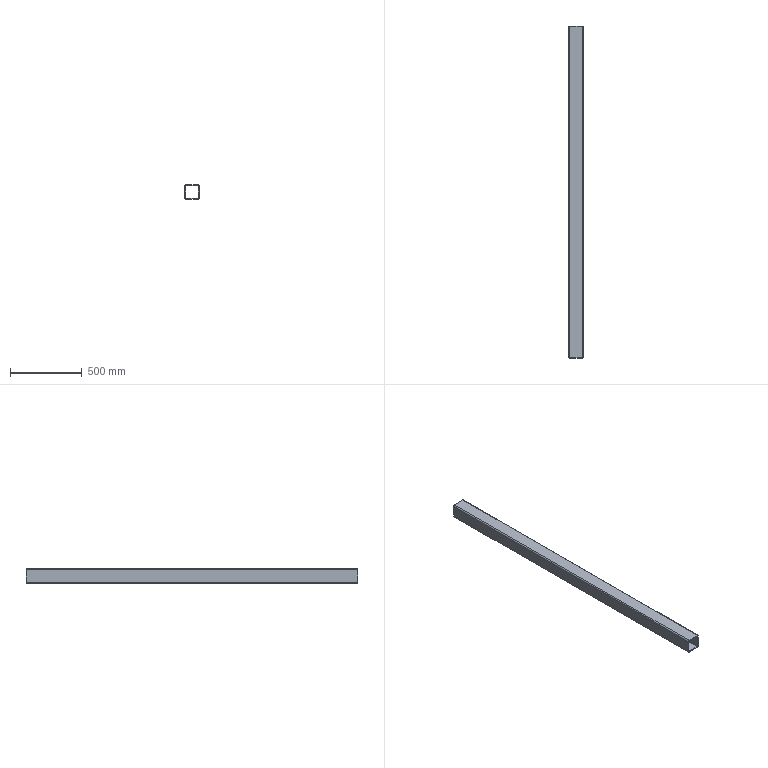Part | SolidWorks | features Extrusion 1 | 1 solid | 18 faces | box 100 x 2320 x 100 mm | volume 5433615 mm3 | plane 10 | cylinder 8 | commonest cylinder face diameters 12.6 x4 15.75 x4
STEP:
#1=CARTESIAN_POINT('',(100.,2320.,-90.6));
#2=VERTEX_POINT('',#1);
#3=CARTESIAN_POINT('',(92.125,2320.,-98.475));
#4=VERTEX_POINT('',#3);
#5=CARTESIAN_POINT('',(92.125,2320.,-90.6));
#6=DIRECTION('',(0.,1.,0.));
#7=DIRECTION('',(0.,0.,1.));
#8=AXIS2_PLACEMENT_3D('',#5,#6,#7);
#9=CIRCLE('',#8,7.875);
#10=EDGE_CURVE('',#2,#4,#9,.T.);
#11=ORIENTED_EDGE('',*,*,#10,.T.);
#12=CARTESIAN_POINT('',(7.875,2320.,-98.475));
#13=VERTEX_POINT('',#12);
#14=CARTESIAN_POINT('',(92.125,2320.,-98.475));
#15=DIRECTION('',(-1.,0.,0.));
#16=VECTOR('',#15,1000.);
#17=LINE('',#14,#16);
#18=EDGE_CURVE('',#4,#13,#17,.T.);
#19=ORIENTED_EDGE('',*,*,#18,.T.);
#20=CARTESIAN_POINT('',(0.,2320.,-90.6));
#21=VERTEX_POINT('',#20);
#22=CARTESIAN_POINT('',(7.875,2320.,-90.6));
#23=DIRECTION('',(0.,1.,0.));
#24=DIRECTION('',(0.,0.,1.));
#25=AXIS2_PLACEMENT_3D('',#22,#23,#24);
#26=CIRCLE('',#25,7.875);
#27=EDGE_CURVE('',#13,#21,#26,.T.);
#28=ORIENTED_EDGE('',*,*,#27,.T.);
#29=CARTESIAN_POINT('',(0.,2320.,-6.35));
#30=VERTEX_POINT('',#29);
#31=CARTESIAN_POINT('',(0.,2320.,-6.35));
#32=DIRECTION('',(0.,0.,1.));
#33=VECTOR('',#32,1000.);
#34=LINE('',#31,#33);
#35=EDGE_CURVE('',#21,#30,#34,.T.);
#36=ORIENTED_EDGE('',*,*,#35,.T.);
#37=CARTESIAN_POINT('',(7.875,2320.,1.525));
#38=VERTEX_POINT('',#37);
#39=CARTESIAN_POINT('',(7.875,2320.,-6.35));
#40=DIRECTION('',(0.,1.,0.));
#41=DIRECTION('',(0.,0.,1.));
#42=AXIS2_PLACEMENT_3D('',#39,#40,#41);
#43=CIRCLE('',#42,7.875);
#44=EDGE_CURVE('',#30,#38,#43,.T.);
#45=ORIENTED_EDGE('',*,*,#44,.T.);
#46=CARTESIAN_POINT('',(92.125,2320.,1.525));
#47=VERTEX_POINT('',#46);
#48=CARTESIAN_POINT('',(7.875,2320.,1.525));
#49=DIRECTION('',(1.,0.,0.));
#50=VECTOR('',#49,1000.);
#51=LINE('',#48,#50);
#52=EDGE_CURVE('',#38,#47,#51,.T.);
#53=ORIENTED_EDGE('',*,*,#52,.T.);
#54=CARTESIAN_POINT('',(100.,2320.,-6.35));
#55=VERTEX_POINT('',#54);
#56=CARTESIAN_POINT('',(92.125,2320.,-6.35));
#57=DIRECTION('',(0.,1.,0.));
#58=DIRECTION('',(0.,0.,1.));
#59=AXIS2_PLACEMENT_3D('',#56,#57,#58);
#60=CIRCLE('',#59,7.875);
#61=EDGE_CURVE('',#47,#55,#60,.T.);
#62=ORIENTED_EDGE('',*,*,#61,.T.);
#63=CARTESIAN_POINT('',(100.,2320.,-90.6));
#64=DIRECTION('',(0.,0.,-1.));
#65=VECTOR('',#64,1000.);
#66=LINE('',#63,#65);
#67=EDGE_CURVE('',#55,#2,#66,.T.);
#68=ORIENTED_EDGE('',*,*,#67,.T.);
#69=EDGE_LOOP('',(#11,#19,#28,#36,#45,#53,#62,#68));
#70=FACE_OUTER_BOUND('',#69,.T.);
#71=CARTESIAN_POINT('',(6.3,2320.,-85.875));
#72=VERTEX_POINT('',#71);
#73=CARTESIAN_POINT('',(6.3,2320.,-11.075));
#74=VERTEX_POINT('',#73);
#75=CARTESIAN_POINT('',(6.3,2320.,-11.075));
#76=DIRECTION('',(0.,0.,1.));
#77=VECTOR('',#76,1000.);
#78=LINE('',#75,#77);
#79=EDGE_CURVE('',#72,#74,#78,.T.);
#80=ORIENTED_EDGE('',*,*,#79,.F.);
#81=CARTESIAN_POINT('',(12.6,2320.,-92.175));
#82=VERTEX_POINT('',#81);
#83=CARTESIAN_POINT('',(12.6,2320.,-85.875));
#84=DIRECTION('',(0.,1.,0.));
#85=DIRECTION('',(0.,0.,1.));
#86=AXIS2_PLACEMENT_3D('',#83,#84,#85);
#87=CIRCLE('',#86,6.3);
#88=EDGE_CURVE('',#82,#72,#87,.T.);
#89=ORIENTED_EDGE('',*,*,#88,.F.);
#90=CARTESIAN_POINT('',(87.4,2320.,-92.175));
#91=VERTEX_POINT('',#90);
#92=CARTESIAN_POINT('',(87.4,2320.,-92.175));
#93=DIRECTION('',(-1.,0.,0.));
#94=VECTOR('',#93,1000.);
#95=LINE('',#92,#94);
#96=EDGE_CURVE('',#91,#82,#95,.T.);
#97=ORIENTED_EDGE('',*,*,#96,.F.);
#98=CARTESIAN_POINT('',(93.7,2320.,-85.875));
#99=VERTEX_POINT('',#98);
#100=CARTESIAN_POINT('',(87.4,2320.,-85.875));
#101=DIRECTION('',(0.,1.,0.));
#102=DIRECTION('',(0.,0.,1.));
#103=AXIS2_PLACEMENT_3D('',#100,#101,#102);
#104=CIRCLE('',#103,6.3);
#105=EDGE_CURVE('',#99,#91,#104,.T.);
#106=ORIENTED_EDGE('',*,*,#105,.F.);
#107=CARTESIAN_POINT('',(93.7,2320.,-11.075));
#108=VERTEX_POINT('',#107);
#109=CARTESIAN_POINT('',(93.7,2320.,-85.875));
#110=DIRECTION('',(0.,0.,-1.));
#111=VECTOR('',#110,1000.);
#112=LINE('',#109,#111);
#113=EDGE_CURVE('',#108,#99,#112,.T.);
#114=ORIENTED_EDGE('',*,*,#113,.F.);
#115=CARTESIAN_POINT('',(87.4,2320.,-4.775));
#116=VERTEX_POINT('',#115);
#117=CARTESIAN_POINT('',(87.4,2320.,-11.075));
#118=DIRECTION('',(0.,1.,0.));
#119=DIRECTION('',(0.,0.,1.));
#120=AXIS2_PLACEMENT_3D('',#117,#118,#119);
#121=CIRCLE('',#120,6.3);
#122=EDGE_CURVE('',#116,#108,#121,.T.);
#123=ORIENTED_EDGE('',*,*,#122,.F.);
#124=CARTESIAN_POINT('',(12.6,2320.,-4.775));
#125=VERTEX_POINT('',#124);
#126=CARTESIAN_POINT('',(12.6,2320.,-4.775));
#127=DIRECTION('',(1.,0.,0.));
#128=VECTOR('',#127,1000.);
#129=LINE('',#126,#128);
#130=EDGE_CURVE('',#125,#116,#129,.T.);
#131=ORIENTED_EDGE('',*,*,#130,.F.);
#132=CARTESIAN_POINT('',(12.6,2320.,-11.075));
#133=DIRECTION('',(0.,1.,0.));
#134=DIRECTION('',(0.,0.,1.));
#135=AXIS2_PLACEMENT_3D('',#132,#133,#134);
#136=CIRCLE('',#135,6.3);
#137=EDGE_CURVE('',#74,#125,#136,.T.);
#138=ORIENTED_EDGE('',*,*,#137,.F.);
#139=EDGE_LOOP('',(#80,#89,#97,#106,#114,#123,#131,#138));
#140=FACE_BOUND('',#139,.T.);
#141=CARTESIAN_POINT('',(92.125,2320.,-90.6));
#142=DIRECTION('',(0.,1.,0.));
#143=DIRECTION('',(0.,0.,1.));
#144=AXIS2_PLACEMENT_3D('',#141,#142,#143);
#145=PLANE('',#144);
#146=ADVANCED_FACE('',(#70,#140),#145,.T.);
#147=CARTESIAN_POINT('',(100.,0.,-90.6));
#148=VERTEX_POINT('',#147);
#149=CARTESIAN_POINT('',(92.125,0.,-98.475));
#150=VERTEX_POINT('',#149);
#151=CARTESIAN_POINT('',(92.125,0.,-90.6));
#152=DIRECTION('',(0.,1.,0.));
#153=DIRECTION('',(0.,0.,1.));
#154=AXIS2_PLACEMENT_3D('',#151,#152,#153);
#155=CIRCLE('',#154,7.875);
#156=EDGE_CURVE('',#148,#150,#155,.T.);
#157=ORIENTED_EDGE('',*,*,#156,.F.);
#158=CARTESIAN_POINT('',(100.,0.,-6.35));
#159=VERTEX_POINT('',#158);
#160=CARTESIAN_POINT('',(100.,0.,-90.6));
#161=DIRECTION('',(0.,0.,-1.));
#162=VECTOR('',#161,1000.);
#163=LINE('',#160,#162);
#164=EDGE_CURVE('',#159,#148,#163,.T.);
#165=ORIENTED_EDGE('',*,*,#164,.F.);
#166=CARTESIAN_POINT('',(92.125,0.,1.525));
#167=VERTEX_POINT('',#166);
#168=CARTESIAN_POINT('',(92.125,0.,-6.35));
#169=DIRECTION('',(0.,1.,0.));
#170=DIRECTION('',(0.,0.,1.));
#171=AXIS2_PLACEMENT_3D('',#168,#169,#170);
#172=CIRCLE('',#171,7.875);
#173=EDGE_CURVE('',#167,#159,#172,.T.);
#174=ORIENTED_EDGE('',*,*,#173,.F.);
#175=CARTESIAN_POINT('',(7.875,0.,1.525));
#176=VERTEX_POINT('',#175);
#177=CARTESIAN_POINT('',(7.875,0.,1.525));
#178=DIRECTION('',(1.,0.,0.));
#179=VECTOR('',#178,1000.);
#180=LINE('',#177,#179);
#181=EDGE_CURVE('',#176,#167,#180,.T.);
#182=ORIENTED_EDGE('',*,*,#181,.F.);
#183=CARTESIAN_POINT('',(0.,0.,-6.35));
#184=VERTEX_POINT('',#183);
#185=CARTESIAN_POINT('',(7.875,0.,-6.35));
#186=DIRECTION('',(0.,1.,0.));
#187=DIRECTION('',(0.,0.,1.));
#188=AXIS2_PLACEMENT_3D('',#185,#186,#187);
#189=CIRCLE('',#188,7.875);
#190=EDGE_CURVE('',#184,#176,#189,.T.);
#191=ORIENTED_EDGE('',*,*,#190,.F.);
#192=CARTESIAN_POINT('',(0.,0.,-90.6));
#193=VERTEX_POINT('',#192);
#194=CARTESIAN_POINT('',(0.,0.,-6.35));
#195=DIRECTION('',(0.,0.,1.));
#196=VECTOR('',#195,1000.);
#197=LINE('',#194,#196);
#198=EDGE_CURVE('',#193,#184,#197,.T.);
#199=ORIENTED_EDGE('',*,*,#198,.F.);
#200=CARTESIAN_POINT('',(7.875,0.,-98.475));
#201=VERTEX_POINT('',#200);
#202=CARTESIAN_POINT('',(7.875,0.,-90.6));
#203=DIRECTION('',(0.,1.,0.));
#204=DIRECTION('',(0.,0.,1.));
#205=AXIS2_PLACEMENT_3D('',#202,#203,#204);
#206=CIRCLE('',#205,7.875);
#207=EDGE_CURVE('',#201,#193,#206,.T.);
#208=ORIENTED_EDGE('',*,*,#207,.F.);
#209=CARTESIAN_POINT('',(92.125,0.,-98.475));
#210=DIRECTION('',(-1.,0.,0.));
#211=VECTOR('',#210,1000.);
#212=LINE('',#209,#211);
#213=EDGE_CURVE('',#150,#201,#212,.T.);
#214=ORIENTED_EDGE('',*,*,#213,.F.);
#215=EDGE_LOOP('',(#157,#165,#174,#182,#191,#199,#208,#214));
#216=FACE_OUTER_BOUND('',#215,.T.);
#217=CARTESIAN_POINT('',(12.6,0.,-92.175));
#218=VERTEX_POINT('',#217);
#219=CARTESIAN_POINT('',(6.3,0.,-85.875));
#220=VERTEX_POINT('',#219);
#221=CARTESIAN_POINT('',(12.6,0.,-85.875));
#222=DIRECTION('',(0.,1.,0.));
#223=DIRECTION('',(0.,0.,1.));
#224=AXIS2_PLACEMENT_3D('',#221,#222,#223);
#225=CIRCLE('',#224,6.3);
#226=EDGE_CURVE('',#218,#220,#225,.T.);
#227=ORIENTED_EDGE('',*,*,#226,.T.);
#228=CARTESIAN_POINT('',(6.3,0.,-11.075));
#229=VERTEX_POINT('',#228);
#230=CARTESIAN_POINT('',(6.3,0.,-11.075));
#231=DIRECTION('',(0.,0.,1.));
#232=VECTOR('',#231,1000.);
#233=LINE('',#230,#232);
#234=EDGE_CURVE('',#220,#229,#233,.T.);
#235=ORIENTED_EDGE('',*,*,#234,.T.);
#236=CARTESIAN_POINT('',(12.6,0.,-4.775));
#237=VERTEX_POINT('',#236);
#238=CARTESIAN_POINT('',(12.6,0.,-11.075));
#239=DIRECTION('',(0.,1.,0.));
#240=DIRECTION('',(0.,0.,1.));
#241=AXIS2_PLACEMENT_3D('',#238,#239,#240);
#242=CIRCLE('',#241,6.3);
#243=EDGE_CURVE('',#229,#237,#242,.T.);
#244=ORIENTED_EDGE('',*,*,#243,.T.);
#245=CARTESIAN_POINT('',(87.4,0.,-4.775));
#246=VERTEX_POINT('',#245);
#247=CARTESIAN_POINT('',(12.6,0.,-4.775));
#248=DIRECTION('',(1.,0.,0.));
#249=VECTOR('',#248,1000.);
#250=LINE('',#247,#249);
#251=EDGE_CURVE('',#237,#246,#250,.T.);
#252=ORIENTED_EDGE('',*,*,#251,.T.);
#253=CARTESIAN_POINT('',(93.7,0.,-11.075));
#254=VERTEX_POINT('',#253);
#255=CARTESIAN_POINT('',(87.4,0.,-11.075));
#256=DIRECTION('',(0.,1.,0.));
#257=DIRECTION('',(0.,0.,1.));
#258=AXIS2_PLACEMENT_3D('',#255,#256,#257);
#259=CIRCLE('',#258,6.3);
#260=EDGE_CURVE('',#246,#254,#259,.T.);
#261=ORIENTED_EDGE('',*,*,#260,.T.);
#262=CARTESIAN_POINT('',(93.7,0.,-85.875));
#263=VERTEX_POINT('',#262);
#264=CARTESIAN_POINT('',(93.7,0.,-85.875));
#265=DIRECTION('',(0.,0.,-1.));
#266=VECTOR('',#265,1000.);
#267=LINE('',#264,#266);
#268=EDGE_CURVE('',#254,#263,#267,.T.);
#269=ORIENTED_EDGE('',*,*,#268,.T.);
#270=CARTESIAN_POINT('',(87.4,0.,-92.175));
#271=VERTEX_POINT('',#270);
#272=CARTESIAN_POINT('',(87.4,0.,-85.875));
#273=DIRECTION('',(0.,1.,0.));
#274=DIRECTION('',(0.,0.,1.));
#275=AXIS2_PLACEMENT_3D('',#272,#273,#274);
#276=CIRCLE('',#275,6.3);
#277=EDGE_CURVE('',#263,#271,#276,.T.);
#278=ORIENTED_EDGE('',*,*,#277,.T.);
#279=CARTESIAN_POINT('',(87.4,0.,-92.175));
#280=DIRECTION('',(-1.,0.,0.));
#281=VECTOR('',#280,1000.);
#282=LINE('',#279,#281);
#283=EDGE_CURVE('',#271,#218,#282,.T.);
#284=ORIENTED_EDGE('',*,*,#283,.T.);
#285=EDGE_LOOP('',(#227,#235,#244,#252,#261,#269,#278,#284));
#286=FACE_BOUND('',#285,.T.);
#287=CARTESIAN_POINT('',(92.125,0.,-90.6));
#288=DIRECTION('',(0.,1.,0.));
#289=DIRECTION('',(0.,0.,1.));
#290=AXIS2_PLACEMENT_3D('',#287,#288,#289);
#291=PLANE('',#290);
#292=ADVANCED_FACE('',(#216,#286),#291,.F.);
#293=ORIENTED_EDGE('',*,*,#156,.T.);
#294=CARTESIAN_POINT('',(92.125,2320.,-98.475));
#295=DIRECTION('',(0.,-1.,0.));
#296=VECTOR('',#295,1000.);
#297=LINE('',#294,#296);
#298=EDGE_CURVE('',#4,#150,#297,.T.);
#299=ORIENTED_EDGE('',*,*,#298,.F.);
#300=ORIENTED_EDGE('',*,*,#10,.F.);
#301=CARTESIAN_POINT('',(100.,2320.,-90.6));
#302=DIRECTION('',(0.,-1.,0.));
#303=VECTOR('',#302,1000.);
#304=LINE('',#301,#303);
#305=EDGE_CURVE('',#2,#148,#304,.T.);
#306=ORIENTED_EDGE('',*,*,#305,.T.);
#307=EDGE_LOOP('',(#293,#299,#300,#306));
#308=FACE_OUTER_BOUND('',#307,.T.);
#309=CARTESIAN_POINT('',(92.125,2320.,-90.6));
#310=DIRECTION('',(0.,-1.,0.));
#311=DIRECTION('',(0.,0.,-1.));
#312=AXIS2_PLACEMENT_3D('',#309,#310,#311);
#313=CYLINDRICAL_SURFACE('',#312,7.875);
#314=ADVANCED_FACE('',(#308),#313,.T.);
#315=ORIENTED_EDGE('',*,*,#213,.T.);
#316=CARTESIAN_POINT('',(7.875,2320.,-98.475));
#317=DIRECTION('',(0.,-1.,0.));
#318=VECTOR('',#317,1000.);
#319=LINE('',#316,#318);
#320=EDGE_CURVE('',#13,#201,#319,.T.);
#321=ORIENTED_EDGE('',*,*,#320,.F.);
#322=ORIENTED_EDGE('',*,*,#18,.F.);
#323=ORIENTED_EDGE('',*,*,#298,.T.);
#324=EDGE_LOOP('',(#315,#321,#322,#323));
#325=FACE_OUTER_BOUND('',#324,.T.);
#326=CARTESIAN_POINT('',(92.125,2320.,-98.475));
#327=DIRECTION('',(0.,0.,1.));
#328=DIRECTION('',(1.,0.,0.));
#329=AXIS2_PLACEMENT_3D('',#326,#327,#328);
#330=PLANE('',#329);
#331=ADVANCED_FACE('',(#325),#330,.F.);
#332=ORIENTED_EDGE('',*,*,#207,.T.);
#333=CARTESIAN_POINT('',(0.,2320.,-90.6));
#334=DIRECTION('',(0.,-1.,0.));
#335=VECTOR('',#334,1000.);
#336=LINE('',#333,#335);
#337=EDGE_CURVE('',#21,#193,#336,.T.);
#338=ORIENTED_EDGE('',*,*,#337,.F.);
#339=ORIENTED_EDGE('',*,*,#27,.F.);
#340=ORIENTED_EDGE('',*,*,#320,.T.);
#341=EDGE_LOOP('',(#332,#338,#339,#340));
#342=FACE_OUTER_BOUND('',#341,.T.);
#343=CARTESIAN_POINT('',(7.875,2320.,-90.6));
#344=DIRECTION('',(0.,-1.,0.));
#345=DIRECTION('',(0.,0.,-1.));
#346=AXIS2_PLACEMENT_3D('',#343,#344,#345);
#347=CYLINDRICAL_SURFACE('',#346,7.875);
#348=ADVANCED_FACE('',(#342),#347,.T.);
#349=ORIENTED_EDGE('',*,*,#198,.T.);
#350=CARTESIAN_POINT('',(0.,2320.,-6.35));
#351=DIRECTION('',(0.,-1.,0.));
#352=VECTOR('',#351,1000.);
#353=LINE('',#350,#352);
#354=EDGE_CURVE('',#30,#184,#353,.T.);
#355=ORIENTED_EDGE('',*,*,#354,.F.);
#356=ORIENTED_EDGE('',*,*,#35,.F.);
#357=ORIENTED_EDGE('',*,*,#337,.T.);
#358=EDGE_LOOP('',(#349,#355,#356,#357));
#359=FACE_OUTER_BOUND('',#358,.T.);
#360=CARTESIAN_POINT('',(0.,2320.,-6.35));
#361=DIRECTION('',(1.,0.,0.));
#362=DIRECTION('',(0.,0.,-1.));
#363=AXIS2_PLACEMENT_3D('',#360,#361,#362);
#364=PLANE('',#363);
#365=ADVANCED_FACE('',(#359),#364,.F.);
#366=ORIENTED_EDGE('',*,*,#190,.T.);
#367=CARTESIAN_POINT('',(7.875,2320.,1.525));
#368=DIRECTION('',(0.,-1.,0.));
#369=VECTOR('',#368,1000.);
#370=LINE('',#367,#369);
#371=EDGE_CURVE('',#38,#176,#370,.T.);
#372=ORIENTED_EDGE('',*,*,#371,.F.);
#373=ORIENTED_EDGE('',*,*,#44,.F.);
#374=ORIENTED_EDGE('',*,*,#354,.T.);
#375=EDGE_LOOP('',(#366,#372,#373,#374));
#376=FACE_OUTER_BOUND('',#375,.T.);
#377=CARTESIAN_POINT('',(7.875,2320.,-6.35));
#378=DIRECTION('',(0.,-1.,0.));
#379=DIRECTION('',(0.,0.,-1.));
#380=AXIS2_PLACEMENT_3D('',#377,#378,#379);
#381=CYLINDRICAL_SURFACE('',#380,7.875);
#382=ADVANCED_FACE('',(#376),#381,.T.);
#383=ORIENTED_EDGE('',*,*,#181,.T.);
#384=CARTESIAN_POINT('',(92.125,2320.,1.525));
#385=DIRECTION('',(0.,-1.,0.));
#386=VECTOR('',#385,1000.);
#387=LINE('',#384,#386);
#388=EDGE_CURVE('',#47,#167,#387,.T.);
#389=ORIENTED_EDGE('',*,*,#388,.F.);
#390=ORIENTED_EDGE('',*,*,#52,.F.);
#391=ORIENTED_EDGE('',*,*,#371,.T.);
#392=EDGE_LOOP('',(#383,#389,#390,#391));
#393=FACE_OUTER_BOUND('',#392,.T.);
#394=CARTESIAN_POINT('',(7.875,2320.,1.525));
#395=DIRECTION('',(0.,0.,-1.));
#396=DIRECTION('',(-1.,0.,0.));
#397=AXIS2_PLACEMENT_3D('',#394,#395,#396);
#398=PLANE('',#397);
#399=ADVANCED_FACE('',(#393),#398,.F.);
#400=ORIENTED_EDGE('',*,*,#173,.T.);
#401=CARTESIAN_POINT('',(100.,2320.,-6.35));
#402=DIRECTION('',(0.,-1.,0.));
#403=VECTOR('',#402,1000.);
#404=LINE('',#401,#403);
#405=EDGE_CURVE('',#55,#159,#404,.T.);
#406=ORIENTED_EDGE('',*,*,#405,.F.);
#407=ORIENTED_EDGE('',*,*,#61,.F.);
#408=ORIENTED_EDGE('',*,*,#388,.T.);
#409=EDGE_LOOP('',(#400,#406,#407,#408));
#410=FACE_OUTER_BOUND('',#409,.T.);
#411=CARTESIAN_POINT('',(92.125,2320.,-6.35));
#412=DIRECTION('',(0.,-1.,0.));
#413=DIRECTION('',(0.,0.,-1.));
#414=AXIS2_PLACEMENT_3D('',#411,#412,#413);
#415=CYLINDRICAL_SURFACE('',#414,7.875);
#416=ADVANCED_FACE('',(#410),#415,.T.);
#417=ORIENTED_EDGE('',*,*,#164,.T.);
#418=ORIENTED_EDGE('',*,*,#305,.F.);
#419=ORIENTED_EDGE('',*,*,#67,.F.);
#420=ORIENTED_EDGE('',*,*,#405,.T.);
#421=EDGE_LOOP('',(#417,#418,#419,#420));
#422=FACE_OUTER_BOUND('',#421,.T.);
#423=CARTESIAN_POINT('',(100.,2320.,-90.6));
#424=DIRECTION('',(-1.,0.,0.));
#425=DIRECTION('',(0.,0.,1.));
#426=AXIS2_PLACEMENT_3D('',#423,#424,#425);
#427=PLANE('',#426);
#428=ADVANCED_FACE('',(#422),#427,.F.);
#429=ORIENTED_EDGE('',*,*,#226,.F.);
#430=CARTESIAN_POINT('',(12.6,2320.,-92.175));
#431=DIRECTION('',(0.,-1.,0.));
#432=VECTOR('',#431,1000.);
#433=LINE('',#430,#432);
#434=EDGE_CURVE('',#82,#218,#433,.T.);
#435=ORIENTED_EDGE('',*,*,#434,.F.);
#436=ORIENTED_EDGE('',*,*,#88,.T.);
#437=CARTESIAN_POINT('',(6.3,2320.,-85.875));
#438=DIRECTION('',(0.,-1.,0.));
#439=VECTOR('',#438,1000.);
#440=LINE('',#437,#439);
#441=EDGE_CURVE('',#72,#220,#440,.T.);
#442=ORIENTED_EDGE('',*,*,#441,.T.);
#443=EDGE_LOOP('',(#429,#435,#436,#442));
#444=FACE_OUTER_BOUND('',#443,.T.);
#445=CARTESIAN_POINT('',(12.6,2320.,-85.875));
#446=DIRECTION('',(0.,-1.,0.));
#447=DIRECTION('',(0.,0.,-1.));
#448=AXIS2_PLACEMENT_3D('',#445,#446,#447);
#449=CYLINDRICAL_SURFACE('',#448,6.3);
#450=ADVANCED_FACE('',(#444),#449,.F.);
#451=ORIENTED_EDGE('',*,*,#234,.F.);
#452=ORIENTED_EDGE('',*,*,#441,.F.);
#453=ORIENTED_EDGE('',*,*,#79,.T.);
#454=CARTESIAN_POINT('',(6.3,2320.,-11.075));
#455=DIRECTION('',(0.,-1.,0.));
#456=VECTOR('',#455,1000.);
#457=LINE('',#454,#456);
#458=EDGE_CURVE('',#74,#229,#457,.T.);
#459=ORIENTED_EDGE('',*,*,#458,.T.);
#460=EDGE_LOOP('',(#451,#452,#453,#459));
#461=FACE_OUTER_BOUND('',#460,.T.);
#462=CARTESIAN_POINT('',(6.3,2320.,-11.075));
#463=DIRECTION('',(1.,0.,0.));
#464=DIRECTION('',(0.,0.,-1.));
#465=AXIS2_PLACEMENT_3D('',#462,#463,#464);
#466=PLANE('',#465);
#467=ADVANCED_FACE('',(#461),#466,.T.);
#468=ORIENTED_EDGE('',*,*,#243,.F.);
#469=ORIENTED_EDGE('',*,*,#458,.F.);
#470=ORIENTED_EDGE('',*,*,#137,.T.);
#471=CARTESIAN_POINT('',(12.6,2320.,-4.775));
#472=DIRECTION('',(0.,-1.,0.));
#473=VECTOR('',#472,1000.);
#474=LINE('',#471,#473);
#475=EDGE_CURVE('',#125,#237,#474,.T.);
#476=ORIENTED_EDGE('',*,*,#475,.T.);
#477=EDGE_LOOP('',(#468,#469,#470,#476));
#478=FACE_OUTER_BOUND('',#477,.T.);
#479=CARTESIAN_POINT('',(12.6,2320.,-11.075));
#480=DIRECTION('',(0.,-1.,0.));
#481=DIRECTION('',(0.,0.,-1.));
#482=AXIS2_PLACEMENT_3D('',#479,#480,#481);
#483=CYLINDRICAL_SURFACE('',#482,6.3);
#484=ADVANCED_FACE('',(#478),#483,.F.);
#485=ORIENTED_EDGE('',*,*,#251,.F.);
#486=ORIENTED_EDGE('',*,*,#475,.F.);
#487=ORIENTED_EDGE('',*,*,#130,.T.);
#488=CARTESIAN_POINT('',(87.4,2320.,-4.775));
#489=DIRECTION('',(0.,-1.,0.));
#490=VECTOR('',#489,1000.);
#491=LINE('',#488,#490);
#492=EDGE_CURVE('',#116,#246,#491,.T.);
#493=ORIENTED_EDGE('',*,*,#492,.T.);
#494=EDGE_LOOP('',(#485,#486,#487,#493));
#495=FACE_OUTER_BOUND('',#494,.T.);
#496=CARTESIAN_POINT('',(12.6,2320.,-4.775));
#497=DIRECTION('',(0.,0.,-1.));
#498=DIRECTION('',(-1.,0.,0.));
#499=AXIS2_PLACEMENT_3D('',#496,#497,#498);
#500=PLANE('',#499);
#501=ADVANCED_FACE('',(#495),#500,.T.);
#502=ORIENTED_EDGE('',*,*,#260,.F.);
#503=ORIENTED_EDGE('',*,*,#492,.F.);
#504=ORIENTED_EDGE('',*,*,#122,.T.);
#505=CARTESIAN_POINT('',(93.7,2320.,-11.075));
#506=DIRECTION('',(0.,-1.,0.));
#507=VECTOR('',#506,1000.);
#508=LINE('',#505,#507);
#509=EDGE_CURVE('',#108,#254,#508,.T.);
#510=ORIENTED_EDGE('',*,*,#509,.T.);
#511=EDGE_LOOP('',(#502,#503,#504,#510));
#512=FACE_OUTER_BOUND('',#511,.T.);
#513=CARTESIAN_POINT('',(87.4,2320.,-11.075));
#514=DIRECTION('',(0.,-1.,0.));
#515=DIRECTION('',(0.,0.,-1.));
#516=AXIS2_PLACEMENT_3D('',#513,#514,#515);
#517=CYLINDRICAL_SURFACE('',#516,6.3);
#518=ADVANCED_FACE('',(#512),#517,.F.);
#519=ORIENTED_EDGE('',*,*,#268,.F.);
#520=ORIENTED_EDGE('',*,*,#509,.F.);
#521=ORIENTED_EDGE('',*,*,#113,.T.);
#522=CARTESIAN_POINT('',(93.7,2320.,-85.875));
#523=DIRECTION('',(0.,-1.,0.));
#524=VECTOR('',#523,1000.);
#525=LINE('',#522,#524);
#526=EDGE_CURVE('',#99,#263,#525,.T.);
#527=ORIENTED_EDGE('',*,*,#526,.T.);
#528=EDGE_LOOP('',(#519,#520,#521,#527));
#529=FACE_OUTER_BOUND('',#528,.T.);
#530=CARTESIAN_POINT('',(93.7,2320.,-85.875));
#531=DIRECTION('',(-1.,0.,0.));
#532=DIRECTION('',(0.,0.,1.));
#533=AXIS2_PLACEMENT_3D('',#530,#531,#532);
#534=PLANE('',#533);
#535=ADVANCED_FACE('',(#529),#534,.T.);
#536=ORIENTED_EDGE('',*,*,#277,.F.);
#537=ORIENTED_EDGE('',*,*,#526,.F.);
#538=ORIENTED_EDGE('',*,*,#105,.T.);
#539=CARTESIAN_POINT('',(87.4,2320.,-92.175));
#540=DIRECTION('',(0.,-1.,0.));
#541=VECTOR('',#540,1000.);
#542=LINE('',#539,#541);
#543=EDGE_CURVE('',#91,#271,#542,.T.);
#544=ORIENTED_EDGE('',*,*,#543,.T.);
#545=EDGE_LOOP('',(#536,#537,#538,#544));
#546=FACE_OUTER_BOUND('',#545,.T.);
#547=CARTESIAN_POINT('',(87.4,2320.,-85.875));
#548=DIRECTION('',(0.,-1.,0.));
#549=DIRECTION('',(0.,0.,-1.));
#550=AXIS2_PLACEMENT_3D('',#547,#548,#549);
#551=CYLINDRICAL_SURFACE('',#550,6.3);
#552=ADVANCED_FACE('',(#546),#551,.F.);
#553=ORIENTED_EDGE('',*,*,#283,.F.);
#554=ORIENTED_EDGE('',*,*,#543,.F.);
#555=ORIENTED_EDGE('',*,*,#96,.T.);
#556=ORIENTED_EDGE('',*,*,#434,.T.);
#557=EDGE_LOOP('',(#553,#554,#555,#556));
#558=FACE_OUTER_BOUND('',#557,.T.);
#559=CARTESIAN_POINT('',(87.4,2320.,-92.175));
#560=DIRECTION('',(0.,0.,1.));
#561=DIRECTION('',(1.,0.,0.));
#562=AXIS2_PLACEMENT_3D('',#559,#560,#561);
#563=PLANE('',#562);
#564=ADVANCED_FACE('',(#558),#563,.T.);
#565=CLOSED_SHELL('',(#146,#292,#314,#331,#348,#365,#382,#399,#416,#428,#450,#467,#484,#501,#518,#535,#552,#564));
#566=MANIFOLD_SOLID_BREP('',#565);
#567=CARTESIAN_POINT('',(0.,0.,0.));
#568=DIRECTION('',(0.,0.,1.));
#569=DIRECTION('',(1.,0.,0.));
#570=AXIS2_PLACEMENT_3D('',#567,#568,#569);
#571=(LENGTH_UNIT()NAMED_UNIT(*)SI_UNIT(.MILLI.,.METRE.));
#572=UNCERTAINTY_MEASURE_WITH_UNIT(LENGTH_MEASURE(0.00001),#571,'','');
#573=(NAMED_UNIT(*)PLANE_ANGLE_UNIT()SI_UNIT($,.RADIAN.));
#574=(NAMED_UNIT(*)SI_UNIT($,.STERADIAN.)SOLID_ANGLE_UNIT());
#575=(GEOMETRIC_REPRESENTATION_CONTEXT(3)GLOBAL_UNCERTAINTY_ASSIGNED_CONTEXT((#572))GLOBAL_UNIT_ASSIGNED_CONTEXT((#571,#573,#574))REPRESENTATION_CONTEXT('',''));
#576=ADVANCED_BREP_SHAPE_REPRESENTATION('',(#566,#570),#575);